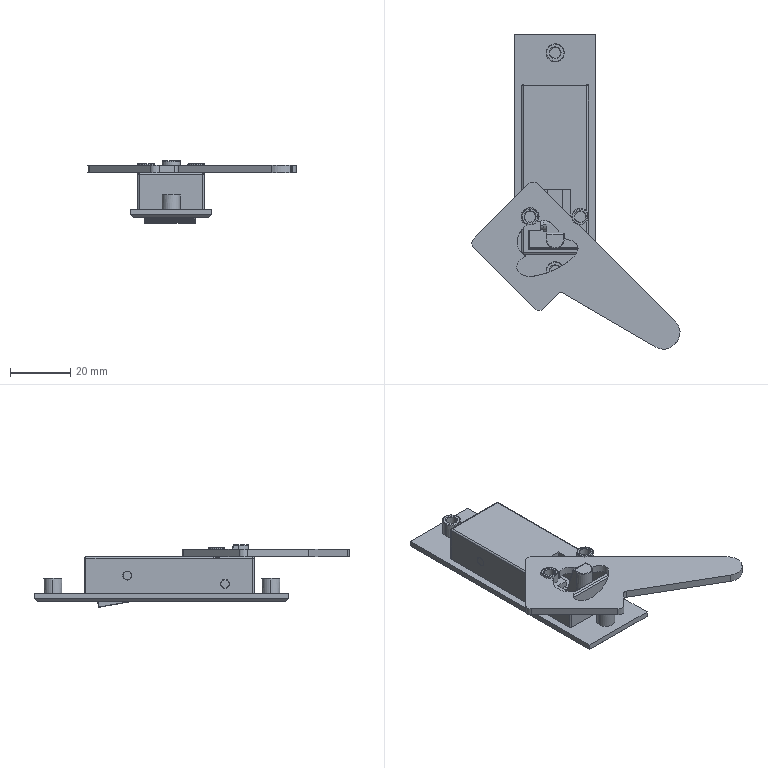Part | SolidWorks | 6 solids | 405 faces | box 69.225 x 104.569 x 20.798 mm | volume 17145 mm3 | plane 238 | cylinder 105 | spline 44 | cone 16 | torus 2 | commonest cylinder face diameters 0.4 x31 3 x16 0.2 x11 1 x11 3.6 x8 4 x8